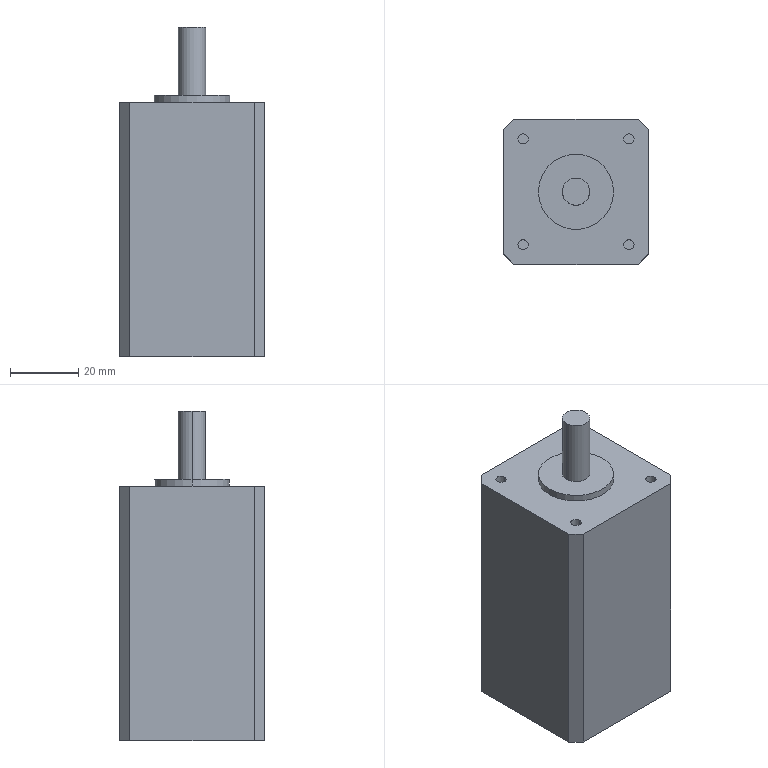Part | SolidWorks | features BaseBody 1 | 1 solid | 28 faces | box 42.3 x 42.3 x 96.5 mm | volume 133444 mm3 | plane 16 | cylinder 12 | commonest cylinder face diameters 3 x8 8 x2 22 x2
STEP:
#1=CARTESIAN_POINT('',(-11.,0.,76.5));
#2=VERTEX_POINT('',#1);
#3=CARTESIAN_POINT('',(11.,0.,76.5));
#4=VERTEX_POINT('',#3);
#5=CARTESIAN_POINT('',(0.,0.,76.5));
#6=DIRECTION('',(0.,0.,-1.));
#7=DIRECTION('',(-1.,0.,0.));
#8=AXIS2_PLACEMENT_3D('',#5,#6,#7);
#9=CIRCLE('',#8,11.);
#10=EDGE_CURVE('',#2,#4,#9,.T.);
#11=ORIENTED_EDGE('',*,*,#10,.T.);
#12=CARTESIAN_POINT('',(11.,0.,74.5));
#13=VERTEX_POINT('',#12);
#14=CARTESIAN_POINT('',(11.,0.,76.5));
#15=DIRECTION('',(0.,0.,-1.));
#16=VECTOR('',#15,1000.);
#17=LINE('',#14,#16);
#18=EDGE_CURVE('',#4,#13,#17,.T.);
#19=ORIENTED_EDGE('',*,*,#18,.T.);
#20=CARTESIAN_POINT('',(-11.,0.,74.5));
#21=VERTEX_POINT('',#20);
#22=CARTESIAN_POINT('',(0.,0.,74.5));
#23=DIRECTION('',(0.,0.,-1.));
#24=DIRECTION('',(-1.,0.,0.));
#25=AXIS2_PLACEMENT_3D('',#22,#23,#24);
#26=CIRCLE('',#25,11.);
#27=EDGE_CURVE('',#21,#13,#26,.T.);
#28=ORIENTED_EDGE('',*,*,#27,.F.);
#29=CARTESIAN_POINT('',(-11.,0.,76.5));
#30=DIRECTION('',(0.,0.,-1.));
#31=VECTOR('',#30,1000.);
#32=LINE('',#29,#31);
#33=EDGE_CURVE('',#2,#21,#32,.T.);
#34=ORIENTED_EDGE('',*,*,#33,.F.);
#35=EDGE_LOOP('',(#11,#19,#28,#34));
#36=FACE_OUTER_BOUND('',#35,.T.);
#37=CARTESIAN_POINT('',(0.,0.,76.5));
#38=DIRECTION('',(0.,0.,-1.));
#39=DIRECTION('',(-1.,0.,0.));
#40=AXIS2_PLACEMENT_3D('',#37,#38,#39);
#41=CYLINDRICAL_SURFACE('',#40,11.);
#42=ADVANCED_FACE('',(#36),#41,.T.);
#43=CARTESIAN_POINT('',(14.,-15.5,64.5));
#44=VERTEX_POINT('',#43);
#45=CARTESIAN_POINT('',(17.,-15.5,64.5));
#46=VERTEX_POINT('',#45);
#47=CARTESIAN_POINT('',(15.5,-15.5,64.5));
#48=DIRECTION('',(0.,0.,1.));
#49=DIRECTION('',(1.,0.,0.));
#50=AXIS2_PLACEMENT_3D('',#47,#48,#49);
#51=CIRCLE('',#50,1.5);
#52=EDGE_CURVE('',#44,#46,#51,.T.);
#53=ORIENTED_EDGE('',*,*,#52,.F.);
#54=CARTESIAN_POINT('',(14.,-15.5,74.5));
#55=VERTEX_POINT('',#54);
#56=CARTESIAN_POINT('',(14.,-15.5,64.5));
#57=DIRECTION('',(0.,0.,1.));
#58=VECTOR('',#57,1000.);
#59=LINE('',#56,#58);
#60=EDGE_CURVE('',#44,#55,#59,.T.);
#61=ORIENTED_EDGE('',*,*,#60,.T.);
#62=CARTESIAN_POINT('',(17.,-15.5,74.5));
#63=VERTEX_POINT('',#62);
#64=CARTESIAN_POINT('',(15.5,-15.5,74.5));
#65=DIRECTION('',(0.,0.,-1.));
#66=DIRECTION('',(1.,0.,0.));
#67=AXIS2_PLACEMENT_3D('',#64,#65,#66);
#68=CIRCLE('',#67,1.5);
#69=EDGE_CURVE('',#63,#55,#68,.T.);
#70=ORIENTED_EDGE('',*,*,#69,.F.);
#71=CARTESIAN_POINT('',(17.,-15.5,64.5));
#72=DIRECTION('',(0.,0.,1.));
#73=VECTOR('',#72,1000.);
#74=LINE('',#71,#73);
#75=EDGE_CURVE('',#46,#63,#74,.T.);
#76=ORIENTED_EDGE('',*,*,#75,.F.);
#77=EDGE_LOOP('',(#53,#61,#70,#76));
#78=FACE_OUTER_BOUND('',#77,.T.);
#79=CARTESIAN_POINT('',(15.5,-15.5,64.5));
#80=DIRECTION('',(0.,0.,1.));
#81=DIRECTION('',(1.,0.,0.));
#82=AXIS2_PLACEMENT_3D('',#79,#80,#81);
#83=CYLINDRICAL_SURFACE('',#82,1.5);
#84=ADVANCED_FACE('',(#78),#83,.F.);
#85=CARTESIAN_POINT('',(-17.,15.5,64.5));
#86=VERTEX_POINT('',#85);
#87=CARTESIAN_POINT('',(-14.,15.5,64.5));
#88=VERTEX_POINT('',#87);
#89=CARTESIAN_POINT('',(-15.5,15.5,64.5));
#90=DIRECTION('',(0.,0.,1.));
#91=DIRECTION('',(1.,0.,0.));
#92=AXIS2_PLACEMENT_3D('',#89,#90,#91);
#93=CIRCLE('',#92,1.5);
#94=EDGE_CURVE('',#86,#88,#93,.T.);
#95=ORIENTED_EDGE('',*,*,#94,.F.);
#96=CARTESIAN_POINT('',(-17.,15.5,74.5));
#97=VERTEX_POINT('',#96);
#98=CARTESIAN_POINT('',(-17.,15.5,64.5));
#99=DIRECTION('',(0.,0.,1.));
#100=VECTOR('',#99,1000.);
#101=LINE('',#98,#100);
#102=EDGE_CURVE('',#86,#97,#101,.T.);
#103=ORIENTED_EDGE('',*,*,#102,.T.);
#104=CARTESIAN_POINT('',(-14.,15.5,74.5));
#105=VERTEX_POINT('',#104);
#106=CARTESIAN_POINT('',(-15.5,15.5,74.5));
#107=DIRECTION('',(0.,0.,-1.));
#108=DIRECTION('',(1.,0.,0.));
#109=AXIS2_PLACEMENT_3D('',#106,#107,#108);
#110=CIRCLE('',#109,1.5);
#111=EDGE_CURVE('',#105,#97,#110,.T.);
#112=ORIENTED_EDGE('',*,*,#111,.F.);
#113=CARTESIAN_POINT('',(-14.,15.5,64.5));
#114=DIRECTION('',(0.,0.,1.));
#115=VECTOR('',#114,1000.);
#116=LINE('',#113,#115);
#117=EDGE_CURVE('',#88,#105,#116,.T.);
#118=ORIENTED_EDGE('',*,*,#117,.F.);
#119=EDGE_LOOP('',(#95,#103,#112,#118));
#120=FACE_OUTER_BOUND('',#119,.T.);
#121=CARTESIAN_POINT('',(-15.5,15.5,64.5));
#122=DIRECTION('',(0.,0.,1.));
#123=DIRECTION('',(1.,0.,0.));
#124=AXIS2_PLACEMENT_3D('',#121,#122,#123);
#125=CYLINDRICAL_SURFACE('',#124,1.5);
#126=ADVANCED_FACE('',(#120),#125,.F.);
#127=CARTESIAN_POINT('',(14.,15.5,64.5));
#128=VERTEX_POINT('',#127);
#129=CARTESIAN_POINT('',(17.,15.5,64.5));
#130=VERTEX_POINT('',#129);
#131=CARTESIAN_POINT('',(15.5,15.5,64.5));
#132=DIRECTION('',(0.,0.,1.));
#133=DIRECTION('',(1.,0.,0.));
#134=AXIS2_PLACEMENT_3D('',#131,#132,#133);
#135=CIRCLE('',#134,1.5);
#136=EDGE_CURVE('',#128,#130,#135,.T.);
#137=ORIENTED_EDGE('',*,*,#136,.F.);
#138=CARTESIAN_POINT('',(14.,15.5,74.5));
#139=VERTEX_POINT('',#138);
#140=CARTESIAN_POINT('',(14.,15.5,64.5));
#141=DIRECTION('',(0.,0.,1.));
#142=VECTOR('',#141,1000.);
#143=LINE('',#140,#142);
#144=EDGE_CURVE('',#128,#139,#143,.T.);
#145=ORIENTED_EDGE('',*,*,#144,.T.);
#146=CARTESIAN_POINT('',(17.,15.5,74.5));
#147=VERTEX_POINT('',#146);
#148=CARTESIAN_POINT('',(15.5,15.5,74.5));
#149=DIRECTION('',(0.,0.,-1.));
#150=DIRECTION('',(1.,0.,0.));
#151=AXIS2_PLACEMENT_3D('',#148,#149,#150);
#152=CIRCLE('',#151,1.5);
#153=EDGE_CURVE('',#147,#139,#152,.T.);
#154=ORIENTED_EDGE('',*,*,#153,.F.);
#155=CARTESIAN_POINT('',(17.,15.5,64.5));
#156=DIRECTION('',(0.,0.,1.));
#157=VECTOR('',#156,1000.);
#158=LINE('',#155,#157);
#159=EDGE_CURVE('',#130,#147,#158,.T.);
#160=ORIENTED_EDGE('',*,*,#159,.F.);
#161=EDGE_LOOP('',(#137,#145,#154,#160));
#162=FACE_OUTER_BOUND('',#161,.T.);
#163=CARTESIAN_POINT('',(15.5,15.5,64.5));
#164=DIRECTION('',(0.,0.,1.));
#165=DIRECTION('',(1.,0.,0.));
#166=AXIS2_PLACEMENT_3D('',#163,#164,#165);
#167=CYLINDRICAL_SURFACE('',#166,1.5);
#168=ADVANCED_FACE('',(#162),#167,.F.);
#169=CARTESIAN_POINT('',(-17.,-15.5,64.5));
#170=VERTEX_POINT('',#169);
#171=CARTESIAN_POINT('',(-14.,-15.5,64.5));
#172=VERTEX_POINT('',#171);
#173=CARTESIAN_POINT('',(-15.5,-15.5,64.5));
#174=DIRECTION('',(0.,0.,1.));
#175=DIRECTION('',(1.,0.,0.));
#176=AXIS2_PLACEMENT_3D('',#173,#174,#175);
#177=CIRCLE('',#176,1.5);
#178=EDGE_CURVE('',#170,#172,#177,.T.);
#179=ORIENTED_EDGE('',*,*,#178,.F.);
#180=CARTESIAN_POINT('',(-17.,-15.5,74.5));
#181=VERTEX_POINT('',#180);
#182=CARTESIAN_POINT('',(-17.,-15.5,64.5));
#183=DIRECTION('',(0.,0.,1.));
#184=VECTOR('',#183,1000.);
#185=LINE('',#182,#184);
#186=EDGE_CURVE('',#170,#181,#185,.T.);
#187=ORIENTED_EDGE('',*,*,#186,.T.);
#188=CARTESIAN_POINT('',(-14.,-15.5,74.5));
#189=VERTEX_POINT('',#188);
#190=CARTESIAN_POINT('',(-15.5,-15.5,74.5));
#191=DIRECTION('',(0.,0.,-1.));
#192=DIRECTION('',(1.,0.,0.));
#193=AXIS2_PLACEMENT_3D('',#190,#191,#192);
#194=CIRCLE('',#193,1.5);
#195=EDGE_CURVE('',#189,#181,#194,.T.);
#196=ORIENTED_EDGE('',*,*,#195,.F.);
#197=CARTESIAN_POINT('',(-14.,-15.5,64.5));
#198=DIRECTION('',(0.,0.,1.));
#199=VECTOR('',#198,1000.);
#200=LINE('',#197,#199);
#201=EDGE_CURVE('',#172,#189,#200,.T.);
#202=ORIENTED_EDGE('',*,*,#201,.F.);
#203=EDGE_LOOP('',(#179,#187,#196,#202));
#204=FACE_OUTER_BOUND('',#203,.T.);
#205=CARTESIAN_POINT('',(-15.5,-15.5,64.5));
#206=DIRECTION('',(0.,0.,1.));
#207=DIRECTION('',(1.,0.,0.));
#208=AXIS2_PLACEMENT_3D('',#205,#206,#207);
#209=CYLINDRICAL_SURFACE('',#208,1.5);
#210=ADVANCED_FACE('',(#204),#209,.F.);
#211=CARTESIAN_POINT('',(-4.,0.,96.5));
#212=VERTEX_POINT('',#211);
#213=CARTESIAN_POINT('',(4.,0.,96.5));
#214=VERTEX_POINT('',#213);
#215=CARTESIAN_POINT('',(0.,0.,96.5));
#216=DIRECTION('',(0.,0.,-1.));
#217=DIRECTION('',(-1.,0.,0.));
#218=AXIS2_PLACEMENT_3D('',#215,#216,#217);
#219=CIRCLE('',#218,4.);
#220=EDGE_CURVE('',#212,#214,#219,.T.);
#221=ORIENTED_EDGE('',*,*,#220,.T.);
#222=CARTESIAN_POINT('',(4.,0.,76.5));
#223=VERTEX_POINT('',#222);
#224=CARTESIAN_POINT('',(4.,0.,96.5));
#225=DIRECTION('',(0.,0.,-1.));
#226=VECTOR('',#225,1000.);
#227=LINE('',#224,#226);
#228=EDGE_CURVE('',#214,#223,#227,.T.);
#229=ORIENTED_EDGE('',*,*,#228,.T.);
#230=CARTESIAN_POINT('',(-4.,0.,76.5));
#231=VERTEX_POINT('',#230);
#232=CARTESIAN_POINT('',(0.,0.,76.5));
#233=DIRECTION('',(0.,0.,-1.));
#234=DIRECTION('',(-1.,0.,0.));
#235=AXIS2_PLACEMENT_3D('',#232,#233,#234);
#236=CIRCLE('',#235,4.);
#237=EDGE_CURVE('',#231,#223,#236,.T.);
#238=ORIENTED_EDGE('',*,*,#237,.F.);
#239=CARTESIAN_POINT('',(-4.,0.,96.5));
#240=DIRECTION('',(0.,0.,-1.));
#241=VECTOR('',#240,1000.);
#242=LINE('',#239,#241);
#243=EDGE_CURVE('',#212,#231,#242,.T.);
#244=ORIENTED_EDGE('',*,*,#243,.F.);
#245=EDGE_LOOP('',(#221,#229,#238,#244));
#246=FACE_OUTER_BOUND('',#245,.T.);
#247=CARTESIAN_POINT('',(0.,0.,96.5));
#248=DIRECTION('',(0.,0.,-1.));
#249=DIRECTION('',(-1.,0.,0.));
#250=AXIS2_PLACEMENT_3D('',#247,#248,#249);
#251=CYLINDRICAL_SURFACE('',#250,4.);
#252=ADVANCED_FACE('',(#246),#251,.T.);
#253=CARTESIAN_POINT('',(18.15,21.15,0.));
#254=VERTEX_POINT('',#253);
#255=CARTESIAN_POINT('',(18.15,21.15,74.5));
#256=VERTEX_POINT('',#255);
#257=CARTESIAN_POINT('',(18.15,21.15,74.5));
#258=DIRECTION('',(0.,0.,1.));
#259=VECTOR('',#258,1000.);
#260=LINE('',#257,#259);
#261=EDGE_CURVE('',#254,#256,#260,.T.);
#262=ORIENTED_EDGE('',*,*,#261,.F.);
#263=CARTESIAN_POINT('',(-18.15,21.15,0.));
#264=VERTEX_POINT('',#263);
#265=CARTESIAN_POINT('',(-21.15,21.15,0.));
#266=DIRECTION('',(1.,0.,0.));
#267=VECTOR('',#266,1000.);
#268=LINE('',#265,#267);
#269=EDGE_CURVE('',#264,#254,#268,.T.);
#270=ORIENTED_EDGE('',*,*,#269,.F.);
#271=CARTESIAN_POINT('',(-18.15,21.15,74.5));
#272=VERTEX_POINT('',#271);
#273=CARTESIAN_POINT('',(-18.15,21.15,74.5));
#274=DIRECTION('',(0.,0.,-1.));
#275=VECTOR('',#274,1000.);
#276=LINE('',#273,#275);
#277=EDGE_CURVE('',#272,#264,#276,.T.);
#278=ORIENTED_EDGE('',*,*,#277,.F.);
#279=CARTESIAN_POINT('',(-21.15,21.15,74.5));
#280=DIRECTION('',(-1.,0.,0.));
#281=VECTOR('',#280,1000.);
#282=LINE('',#279,#281);
#283=EDGE_CURVE('',#256,#272,#282,.T.);
#284=ORIENTED_EDGE('',*,*,#283,.F.);
#285=EDGE_LOOP('',(#262,#270,#278,#284));
#286=FACE_OUTER_BOUND('',#285,.T.);
#287=CARTESIAN_POINT('',(-21.15,21.15,74.5));
#288=DIRECTION('',(0.,-1.,0.));
#289=DIRECTION('',(0.,0.,-1.));
#290=AXIS2_PLACEMENT_3D('',#287,#288,#289);
#291=PLANE('',#290);
#292=ADVANCED_FACE('',(#286),#291,.F.);
#293=CARTESIAN_POINT('',(-18.15,-21.15,74.5));
#294=VERTEX_POINT('',#293);
#295=CARTESIAN_POINT('',(18.15,-21.15,74.5));
#296=VERTEX_POINT('',#295);
#297=CARTESIAN_POINT('',(0.,-21.15,74.5));
#298=DIRECTION('',(1.,0.,0.));
#299=VECTOR('',#298,1000.);
#300=LINE('',#297,#299);
#301=EDGE_CURVE('',#294,#296,#300,.T.);
#302=ORIENTED_EDGE('',*,*,#301,.T.);
#303=CARTESIAN_POINT('',(21.15,-18.15,74.5));
#304=VERTEX_POINT('',#303);
#305=CARTESIAN_POINT('',(18.15,-21.15,74.5));
#306=DIRECTION('',(0.7071,0.7071,0.));
#307=VECTOR('',#306,1000.);
#308=LINE('',#305,#307);
#309=EDGE_CURVE('',#296,#304,#308,.T.);
#310=ORIENTED_EDGE('',*,*,#309,.T.);
#311=CARTESIAN_POINT('',(21.15,18.15,74.5));
#312=VERTEX_POINT('',#311);
#313=CARTESIAN_POINT('',(21.15,0.,74.5));
#314=DIRECTION('',(0.,1.,0.));
#315=VECTOR('',#314,1000.);
#316=LINE('',#313,#315);
#317=EDGE_CURVE('',#304,#312,#316,.T.);
#318=ORIENTED_EDGE('',*,*,#317,.T.);
#319=CARTESIAN_POINT('',(21.15,18.15,74.5));
#320=DIRECTION('',(-0.7071,0.7071,0.));
#321=VECTOR('',#320,1000.);
#322=LINE('',#319,#321);
#323=EDGE_CURVE('',#312,#256,#322,.T.);
#324=ORIENTED_EDGE('',*,*,#323,.T.);
#325=ORIENTED_EDGE('',*,*,#283,.T.);
#326=CARTESIAN_POINT('',(-21.15,18.15,74.5));
#327=VERTEX_POINT('',#326);
#328=CARTESIAN_POINT('',(-18.15,21.15,74.5));
#329=DIRECTION('',(-0.7071,-0.7071,0.));
#330=VECTOR('',#329,1000.);
#331=LINE('',#328,#330);
#332=EDGE_CURVE('',#272,#327,#331,.T.);
#333=ORIENTED_EDGE('',*,*,#332,.T.);
#334=CARTESIAN_POINT('',(-21.15,-18.15,74.5));
#335=VERTEX_POINT('',#334);
#336=CARTESIAN_POINT('',(-21.15,0.,74.5));
#337=DIRECTION('',(0.,-1.,0.));
#338=VECTOR('',#337,1000.);
#339=LINE('',#336,#338);
#340=EDGE_CURVE('',#327,#335,#339,.T.);
#341=ORIENTED_EDGE('',*,*,#340,.T.);
#342=CARTESIAN_POINT('',(-21.15,-18.15,74.5));
#343=DIRECTION('',(0.7071,-0.7071,0.));
#344=VECTOR('',#343,1000.);
#345=LINE('',#342,#344);
#346=EDGE_CURVE('',#335,#294,#345,.T.);
#347=ORIENTED_EDGE('',*,*,#346,.T.);
#348=EDGE_LOOP('',(#302,#310,#318,#324,#325,#333,#341,#347));
#349=FACE_OUTER_BOUND('',#348,.T.);
#350=ORIENTED_EDGE('',*,*,#27,.T.);
#351=CARTESIAN_POINT('',(0.,0.,74.5));
#352=DIRECTION('',(0.,0.,-1.));
#353=DIRECTION('',(-1.,0.,0.));
#354=AXIS2_PLACEMENT_3D('',#351,#352,#353);
#355=CIRCLE('',#354,11.);
#356=EDGE_CURVE('',#13,#21,#355,.T.);
#357=ORIENTED_EDGE('',*,*,#356,.T.);
#358=EDGE_LOOP('',(#350,#357));
#359=FACE_BOUND('',#358,.T.);
#360=ORIENTED_EDGE('',*,*,#69,.T.);
#361=CARTESIAN_POINT('',(15.5,-15.5,74.5));
#362=DIRECTION('',(0.,0.,-1.));
#363=DIRECTION('',(1.,0.,0.));
#364=AXIS2_PLACEMENT_3D('',#361,#362,#363);
#365=CIRCLE('',#364,1.5);
#366=EDGE_CURVE('',#55,#63,#365,.T.);
#367=ORIENTED_EDGE('',*,*,#366,.T.);
#368=EDGE_LOOP('',(#360,#367));
#369=FACE_BOUND('',#368,.T.);
#370=ORIENTED_EDGE('',*,*,#111,.T.);
#371=CARTESIAN_POINT('',(-15.5,15.5,74.5));
#372=DIRECTION('',(0.,0.,-1.));
#373=DIRECTION('',(1.,0.,0.));
#374=AXIS2_PLACEMENT_3D('',#371,#372,#373);
#375=CIRCLE('',#374,1.5);
#376=EDGE_CURVE('',#97,#105,#375,.T.);
#377=ORIENTED_EDGE('',*,*,#376,.T.);
#378=EDGE_LOOP('',(#370,#377));
#379=FACE_BOUND('',#378,.T.);
#380=ORIENTED_EDGE('',*,*,#153,.T.);
#381=CARTESIAN_POINT('',(15.5,15.5,74.5));
#382=DIRECTION('',(0.,0.,-1.));
#383=DIRECTION('',(1.,0.,0.));
#384=AXIS2_PLACEMENT_3D('',#381,#382,#383);
#385=CIRCLE('',#384,1.5);
#386=EDGE_CURVE('',#139,#147,#385,.T.);
#387=ORIENTED_EDGE('',*,*,#386,.T.);
#388=EDGE_LOOP('',(#380,#387));
#389=FACE_BOUND('',#388,.T.);
#390=ORIENTED_EDGE('',*,*,#195,.T.);
#391=CARTESIAN_POINT('',(-15.5,-15.5,74.5));
#392=DIRECTION('',(0.,0.,-1.));
#393=DIRECTION('',(1.,0.,0.));
#394=AXIS2_PLACEMENT_3D('',#391,#392,#393);
#395=CIRCLE('',#394,1.5);
#396=EDGE_CURVE('',#181,#189,#395,.T.);
#397=ORIENTED_EDGE('',*,*,#396,.T.);
#398=EDGE_LOOP('',(#390,#397));
#399=FACE_BOUND('',#398,.T.);
#400=CARTESIAN_POINT('',(0.,0.,74.5));
#401=DIRECTION('',(0.,0.,1.));
#402=DIRECTION('',(1.,0.,0.));
#403=AXIS2_PLACEMENT_3D('',#400,#401,#402);
#404=PLANE('',#403);
#405=ADVANCED_FACE('',(#349,#359,#369,#379,#389,#399),#404,.T.);
#406=CARTESIAN_POINT('',(21.15,18.15,0.));
#407=VERTEX_POINT('',#406);
#408=CARTESIAN_POINT('',(21.15,18.15,74.5));
#409=DIRECTION('',(0.,0.,1.));
#410=VECTOR('',#409,1000.);
#411=LINE('',#408,#410);
#412=EDGE_CURVE('',#407,#312,#411,.T.);
#413=ORIENTED_EDGE('',*,*,#412,.F.);
#414=CARTESIAN_POINT('',(18.15,21.15,0.));
#415=DIRECTION('',(0.7071,-0.7071,0.));
#416=VECTOR('',#415,1000.);
#417=LINE('',#414,#416);
#418=EDGE_CURVE('',#254,#407,#417,.T.);
#419=ORIENTED_EDGE('',*,*,#418,.F.);
#420=ORIENTED_EDGE('',*,*,#261,.T.);
#421=ORIENTED_EDGE('',*,*,#323,.F.);
#422=EDGE_LOOP('',(#413,#419,#420,#421));
#423=FACE_OUTER_BOUND('',#422,.T.);
#424=CARTESIAN_POINT('',(18.15,21.15,74.5));
#425=DIRECTION('',(-0.7071,-0.7071,0.));
#426=DIRECTION('',(0.7071,-0.7071,0.));
#427=AXIS2_PLACEMENT_3D('',#424,#425,#426);
#428=PLANE('',#427);
#429=ADVANCED_FACE('',(#423),#428,.F.);
#430=ORIENTED_EDGE('',*,*,#418,.T.);
#431=CARTESIAN_POINT('',(21.15,-18.15,0.));
#432=VERTEX_POINT('',#431);
#433=CARTESIAN_POINT('',(21.15,0.,0.));
#434=DIRECTION('',(0.,1.,0.));
#435=VECTOR('',#434,1000.);
#436=LINE('',#433,#435);
#437=EDGE_CURVE('',#432,#407,#436,.T.);
#438=ORIENTED_EDGE('',*,*,#437,.F.);
#439=CARTESIAN_POINT('',(18.15,-21.15,0.));
#440=VERTEX_POINT('',#439);
#441=CARTESIAN_POINT('',(18.15,-21.15,0.));
#442=DIRECTION('',(0.7071,0.7071,0.));
#443=VECTOR('',#442,1000.);
#444=LINE('',#441,#443);
#445=EDGE_CURVE('',#440,#432,#444,.T.);
#446=ORIENTED_EDGE('',*,*,#445,.F.);
#447=CARTESIAN_POINT('',(-18.15,-21.15,0.));
#448=VERTEX_POINT('',#447);
#449=CARTESIAN_POINT('',(0.,-21.15,0.));
#450=DIRECTION('',(1.,0.,0.));
#451=VECTOR('',#450,1000.);
#452=LINE('',#449,#451);
#453=EDGE_CURVE('',#448,#440,#452,.T.);
#454=ORIENTED_EDGE('',*,*,#453,.F.);
#455=CARTESIAN_POINT('',(-21.15,-18.15,0.));
#456=VERTEX_POINT('',#455);
#457=CARTESIAN_POINT('',(-21.15,-18.15,0.));
#458=DIRECTION('',(0.7071,-0.7071,0.));
#459=VECTOR('',#458,1000.);
#460=LINE('',#457,#459);
#461=EDGE_CURVE('',#456,#448,#460,.T.);
#462=ORIENTED_EDGE('',*,*,#461,.F.);
#463=CARTESIAN_POINT('',(-21.15,18.15,0.));
#464=VERTEX_POINT('',#463);
#465=CARTESIAN_POINT('',(-21.15,0.,0.));
#466=DIRECTION('',(0.,-1.,0.));
#467=VECTOR('',#466,1000.);
#468=LINE('',#465,#467);
#469=EDGE_CURVE('',#464,#456,#468,.T.);
#470=ORIENTED_EDGE('',*,*,#469,.F.);
#471=CARTESIAN_POINT('',(-18.15,21.15,0.));
#472=DIRECTION('',(-0.7071,-0.7071,0.));
#473=VECTOR('',#472,1000.);
#474=LINE('',#471,#473);
#475=EDGE_CURVE('',#264,#464,#474,.T.);
#476=ORIENTED_EDGE('',*,*,#475,.F.);
#477=ORIENTED_EDGE('',*,*,#269,.T.);
#478=EDGE_LOOP('',(#430,#438,#446,#454,#462,#470,#476,#477));
#479=FACE_OUTER_BOUND('',#478,.T.);
#480=CARTESIAN_POINT('',(0.,0.,0.));
#481=DIRECTION('',(0.,0.,1.));
#482=DIRECTION('',(1.,0.,0.));
#483=AXIS2_PLACEMENT_3D('',#480,#481,#482);
#484=PLANE('',#483);
#485=ADVANCED_FACE('',(#479),#484,.F.);
#486=ORIENTED_EDGE('',*,*,#277,.T.);
#487=ORIENTED_EDGE('',*,*,#475,.T.);
#488=CARTESIAN_POINT('',(-21.15,18.15,74.5));
#489=DIRECTION('',(0.,0.,-1.));
#490=VECTOR('',#489,1000.);
#491=LINE('',#488,#490);
#492=EDGE_CURVE('',#327,#464,#491,.T.);
#493=ORIENTED_EDGE('',*,*,#492,.F.);
#494=ORIENTED_EDGE('',*,*,#332,.F.);
#495=EDGE_LOOP('',(#486,#487,#493,#494));
#496=FACE_OUTER_BOUND('',#495,.T.);
#497=CARTESIAN_POINT('',(-21.15,18.15,74.5));
#498=DIRECTION('',(0.7071,-0.7071,0.));
#499=DIRECTION('',(0.7071,0.7071,0.));
#500=AXIS2_PLACEMENT_3D('',#497,#498,#499);
#501=PLANE('',#500);
#502=ADVANCED_FACE('',(#496),#501,.F.);
#503=CARTESIAN_POINT('',(18.15,-21.15,74.5));
#504=DIRECTION('',(0.,0.,1.));
#505=VECTOR('',#504,1000.);
#506=LINE('',#503,#505);
#507=EDGE_CURVE('',#440,#296,#506,.T.);
#508=ORIENTED_EDGE('',*,*,#507,.F.);
#509=ORIENTED_EDGE('',*,*,#445,.T.);
#510=CARTESIAN_POINT('',(21.15,-18.15,74.5));
#511=DIRECTION('',(0.,0.,-1.));
#512=VECTOR('',#511,1000.);
#513=LINE('',#510,#512);
#514=EDGE_CURVE('',#304,#432,#513,.T.);
#515=ORIENTED_EDGE('',*,*,#514,.F.);
#516=ORIENTED_EDGE('',*,*,#309,.F.);
#517=EDGE_LOOP('',(#508,#509,#515,#516));
#518=FACE_OUTER_BOUND('',#517,.T.);
#519=CARTESIAN_POINT('',(21.15,-18.15,74.5));
#520=DIRECTION('',(-0.7071,0.7071,0.));
#521=DIRECTION('',(-0.7071,-0.7071,0.));
#522=AXIS2_PLACEMENT_3D('',#519,#520,#521);
#523=PLANE('',#522);
#524=ADVANCED_FACE('',(#518),#523,.F.);
#525=ORIENTED_EDGE('',*,*,#507,.T.);
#526=ORIENTED_EDGE('',*,*,#301,.F.);
#527=CARTESIAN_POINT('',(-18.15,-21.15,74.5));
#528=DIRECTION('',(0.,0.,1.));
#529=VECTOR('',#528,1000.);
#530=LINE('',#527,#529);
#531=EDGE_CURVE('',#448,#294,#530,.T.);
#532=ORIENTED_EDGE('',*,*,#531,.F.);
#533=ORIENTED_EDGE('',*,*,#453,.T.);
#534=EDGE_LOOP('',(#525,#526,#532,#533));
#535=FACE_OUTER_BOUND('',#534,.T.);
#536=CARTESIAN_POINT('',(-21.15,-21.15,74.5));
#537=DIRECTION('',(0.,1.,0.));
#538=DIRECTION('',(0.,0.,1.));
#539=AXIS2_PLACEMENT_3D('',#536,#537,#538);
#540=PLANE('',#539);
#541=ADVANCED_FACE('',(#535),#540,.F.);
#542=CARTESIAN_POINT('',(-21.15,-18.15,74.5));
#543=DIRECTION('',(0.,0.,1.));
#544=VECTOR('',#543,1000.);
#545=LINE('',#542,#544);
#546=EDGE_CURVE('',#456,#335,#545,.T.);
#547=ORIENTED_EDGE('',*,*,#546,.F.);
#548=ORIENTED_EDGE('',*,*,#461,.T.);
#549=ORIENTED_EDGE('',*,*,#531,.T.);
#550=ORIENTED_EDGE('',*,*,#346,.F.);
#551=EDGE_LOOP('',(#547,#548,#549,#550));
#552=FACE_OUTER_BOUND('',#551,.T.);
#553=CARTESIAN_POINT('',(-18.15,-21.15,74.5));
#554=DIRECTION('',(0.7071,0.7071,0.));
#555=DIRECTION('',(-0.7071,0.7071,0.));
#556=AXIS2_PLACEMENT_3D('',#553,#554,#555);
#557=PLANE('',#556);
#558=ADVANCED_FACE('',(#552),#557,.F.);
#559=ORIENTED_EDGE('',*,*,#492,.T.);
#560=ORIENTED_EDGE('',*,*,#469,.T.);
#561=ORIENTED_EDGE('',*,*,#546,.T.);
#562=ORIENTED_EDGE('',*,*,#340,.F.);
#563=EDGE_LOOP('',(#559,#560,#561,#562));
#564=FACE_OUTER_BOUND('',#563,.T.);
#565=CARTESIAN_POINT('',(-21.15,21.15,74.5));
#566=DIRECTION('',(1.,0.,0.));
#567=DIRECTION('',(0.,1.,0.));
#568=AXIS2_PLACEMENT_3D('',#565,#566,#567);
#569=PLANE('',#568);
#570=ADVANCED_FACE('',(#564),#569,.F.);
#571=ORIENTED_EDGE('',*,*,#412,.T.);
#572=ORIENTED_EDGE('',*,*,#317,.F.);
#573=ORIENTED_EDGE('',*,*,#514,.T.);
#574=ORIENTED_EDGE('',*,*,#437,.T.);
#575=EDGE_LOOP('',(#571,#572,#573,#574));
#576=FACE_OUTER_BOUND('',#575,.T.);
#577=CARTESIAN_POINT('',(21.15,21.15,74.5));
#578=DIRECTION('',(-1.,0.,0.));
#579=DIRECTION('',(0.,-1.,0.));
#580=AXIS2_PLACEMENT_3D('',#577,#578,#579);
#581=PLANE('',#580);
#582=ADVANCED_FACE('',(#576),#581,.F.);
#583=ORIENTED_EDGE('',*,*,#18,.F.);
#584=CARTESIAN_POINT('',(0.,0.,76.5));
#585=DIRECTION('',(0.,0.,-1.));
#586=DIRECTION('',(-1.,0.,0.));
#587=AXIS2_PLACEMENT_3D('',#584,#585,#586);
#588=CIRCLE('',#587,11.);
#589=EDGE_CURVE('',#4,#2,#588,.T.);
#590=ORIENTED_EDGE('',*,*,#589,.T.);
#591=ORIENTED_EDGE('',*,*,#33,.T.);
#592=ORIENTED_EDGE('',*,*,#356,.F.);
#593=EDGE_LOOP('',(#583,#590,#591,#592));
#594=FACE_OUTER_BOUND('',#593,.T.);
#595=CARTESIAN_POINT('',(0.,0.,76.5));
#596=DIRECTION('',(0.,0.,-1.));
#597=DIRECTION('',(-1.,0.,0.));
#598=AXIS2_PLACEMENT_3D('',#595,#596,#597);
#599=CYLINDRICAL_SURFACE('',#598,11.);
#600=ADVANCED_FACE('',(#594),#599,.T.);
#601=ORIENTED_EDGE('',*,*,#60,.F.);
#602=CARTESIAN_POINT('',(15.5,-15.5,64.5));
#603=DIRECTION('',(0.,0.,1.));
#604=DIRECTION('',(1.,0.,0.));
#605=AXIS2_PLACEMENT_3D('',#602,#603,#604);
#606=CIRCLE('',#605,1.5);
#607=EDGE_CURVE('',#46,#44,#606,.T.);
#608=ORIENTED_EDGE('',*,*,#607,.F.);
#609=ORIENTED_EDGE('',*,*,#75,.T.);
#610=ORIENTED_EDGE('',*,*,#366,.F.);
#611=EDGE_LOOP('',(#601,#608,#609,#610));
#612=FACE_OUTER_BOUND('',#611,.T.);
#613=CARTESIAN_POINT('',(15.5,-15.5,64.5));
#614=DIRECTION('',(0.,0.,1.));
#615=DIRECTION('',(1.,0.,0.));
#616=AXIS2_PLACEMENT_3D('',#613,#614,#615);
#617=CYLINDRICAL_SURFACE('',#616,1.5);
#618=ADVANCED_FACE('',(#612),#617,.F.);
#619=ORIENTED_EDGE('',*,*,#102,.F.);
#620=CARTESIAN_POINT('',(-15.5,15.5,64.5));
#621=DIRECTION('',(0.,0.,1.));
#622=DIRECTION('',(1.,0.,0.));
#623=AXIS2_PLACEMENT_3D('',#620,#621,#622);
#624=CIRCLE('',#623,1.5);
#625=EDGE_CURVE('',#88,#86,#624,.T.);
#626=ORIENTED_EDGE('',*,*,#625,.F.);
#627=ORIENTED_EDGE('',*,*,#117,.T.);
#628=ORIENTED_EDGE('',*,*,#376,.F.);
#629=EDGE_LOOP('',(#619,#626,#627,#628));
#630=FACE_OUTER_BOUND('',#629,.T.);
#631=CARTESIAN_POINT('',(-15.5,15.5,64.5));
#632=DIRECTION('',(0.,0.,1.));
#633=DIRECTION('',(1.,0.,0.));
#634=AXIS2_PLACEMENT_3D('',#631,#632,#633);
#635=CYLINDRICAL_SURFACE('',#634,1.5);
#636=ADVANCED_FACE('',(#630),#635,.F.);
#637=ORIENTED_EDGE('',*,*,#144,.F.);
#638=CARTESIAN_POINT('',(15.5,15.5,64.5));
#639=DIRECTION('',(0.,0.,1.));
#640=DIRECTION('',(1.,0.,0.));
#641=AXIS2_PLACEMENT_3D('',#638,#639,#640);
#642=CIRCLE('',#641,1.5);
#643=EDGE_CURVE('',#130,#128,#642,.T.);
#644=ORIENTED_EDGE('',*,*,#643,.F.);
#645=ORIENTED_EDGE('',*,*,#159,.T.);
#646=ORIENTED_EDGE('',*,*,#386,.F.);
#647=EDGE_LOOP('',(#637,#644,#645,#646));
#648=FACE_OUTER_BOUND('',#647,.T.);
#649=CARTESIAN_POINT('',(15.5,15.5,64.5));
#650=DIRECTION('',(0.,0.,1.));
#651=DIRECTION('',(1.,0.,0.));
#652=AXIS2_PLACEMENT_3D('',#649,#650,#651);
#653=CYLINDRICAL_SURFACE('',#652,1.5);
#654=ADVANCED_FACE('',(#648),#653,.F.);
#655=ORIENTED_EDGE('',*,*,#186,.F.);
#656=CARTESIAN_POINT('',(-15.5,-15.5,64.5));
#657=DIRECTION('',(0.,0.,1.));
#658=DIRECTION('',(1.,0.,0.));
#659=AXIS2_PLACEMENT_3D('',#656,#657,#658);
#660=CIRCLE('',#659,1.5);
#661=EDGE_CURVE('',#172,#170,#660,.T.);
#662=ORIENTED_EDGE('',*,*,#661,.F.);
#663=ORIENTED_EDGE('',*,*,#201,.T.);
#664=ORIENTED_EDGE('',*,*,#396,.F.);
#665=EDGE_LOOP('',(#655,#662,#663,#664));
#666=FACE_OUTER_BOUND('',#665,.T.);
#667=CARTESIAN_POINT('',(-15.5,-15.5,64.5));
#668=DIRECTION('',(0.,0.,1.));
#669=DIRECTION('',(1.,0.,0.));
#670=AXIS2_PLACEMENT_3D('',#667,#668,#669);
#671=CYLINDRICAL_SURFACE('',#670,1.5);
#672=ADVANCED_FACE('',(#666),#671,.F.);
#673=ORIENTED_EDGE('',*,*,#10,.F.);
#674=ORIENTED_EDGE('',*,*,#589,.F.);
#675=EDGE_LOOP('',(#673,#674));
#676=FACE_OUTER_BOUND('',#675,.T.);
#677=ORIENTED_EDGE('',*,*,#237,.T.);
#678=CARTESIAN_POINT('',(0.,0.,76.5));
#679=DIRECTION('',(0.,0.,-1.));
#680=DIRECTION('',(-1.,0.,0.));
#681=AXIS2_PLACEMENT_3D('',#678,#679,#680);
#682=CIRCLE('',#681,4.);
#683=EDGE_CURVE('',#223,#231,#682,.T.);
#684=ORIENTED_EDGE('',*,*,#683,.T.);
#685=EDGE_LOOP('',(#677,#684));
#686=FACE_BOUND('',#685,.T.);
#687=CARTESIAN_POINT('',(0.,0.,76.5));
#688=DIRECTION('',(0.,0.,1.));
#689=DIRECTION('',(1.,0.,0.));
#690=AXIS2_PLACEMENT_3D('',#687,#688,#689);
#691=PLANE('',#690);
#692=ADVANCED_FACE('',(#676,#686),#691,.T.);
#693=ORIENTED_EDGE('',*,*,#607,.T.);
#694=ORIENTED_EDGE('',*,*,#52,.T.);
#695=EDGE_LOOP('',(#693,#694));
#696=FACE_OUTER_BOUND('',#695,.T.);
#697=CARTESIAN_POINT('',(15.5,-15.5,64.5));
#698=DIRECTION('',(0.,0.,1.));
#699=DIRECTION('',(1.,0.,0.));
#700=AXIS2_PLACEMENT_3D('',#697,#698,#699);
#701=PLANE('',#700);
#702=ADVANCED_FACE('',(#696),#701,.T.);
#703=ORIENTED_EDGE('',*,*,#625,.T.);
#704=ORIENTED_EDGE('',*,*,#94,.T.);
#705=EDGE_LOOP('',(#703,#704));
#706=FACE_OUTER_BOUND('',#705,.T.);
#707=CARTESIAN_POINT('',(-15.5,15.5,64.5));
#708=DIRECTION('',(0.,0.,1.));
#709=DIRECTION('',(1.,0.,0.));
#710=AXIS2_PLACEMENT_3D('',#707,#708,#709);
#711=PLANE('',#710);
#712=ADVANCED_FACE('',(#706),#711,.T.);
#713=ORIENTED_EDGE('',*,*,#643,.T.);
#714=ORIENTED_EDGE('',*,*,#136,.T.);
#715=EDGE_LOOP('',(#713,#714));
#716=FACE_OUTER_BOUND('',#715,.T.);
#717=CARTESIAN_POINT('',(15.5,15.5,64.5));
#718=DIRECTION('',(0.,0.,1.));
#719=DIRECTION('',(1.,0.,0.));
#720=AXIS2_PLACEMENT_3D('',#717,#718,#719);
#721=PLANE('',#720);
#722=ADVANCED_FACE('',(#716),#721,.T.);
#723=ORIENTED_EDGE('',*,*,#661,.T.);
#724=ORIENTED_EDGE('',*,*,#178,.T.);
#725=EDGE_LOOP('',(#723,#724));
#726=FACE_OUTER_BOUND('',#725,.T.);
#727=CARTESIAN_POINT('',(-15.5,-15.5,64.5));
#728=DIRECTION('',(0.,0.,1.));
#729=DIRECTION('',(1.,0.,0.));
#730=AXIS2_PLACEMENT_3D('',#727,#728,#729);
#731=PLANE('',#730);
#732=ADVANCED_FACE('',(#726),#731,.T.);
#733=ORIENTED_EDGE('',*,*,#228,.F.);
#734=CARTESIAN_POINT('',(0.,0.,96.5));
#735=DIRECTION('',(0.,0.,-1.));
#736=DIRECTION('',(-1.,0.,0.));
#737=AXIS2_PLACEMENT_3D('',#734,#735,#736);
#738=CIRCLE('',#737,4.);
#739=EDGE_CURVE('',#214,#212,#738,.T.);
#740=ORIENTED_EDGE('',*,*,#739,.T.);
#741=ORIENTED_EDGE('',*,*,#243,.T.);
#742=ORIENTED_EDGE('',*,*,#683,.F.);
#743=EDGE_LOOP('',(#733,#740,#741,#742));
#744=FACE_OUTER_BOUND('',#743,.T.);
#745=CARTESIAN_POINT('',(0.,0.,96.5));
#746=DIRECTION('',(0.,0.,-1.));
#747=DIRECTION('',(-1.,0.,0.));
#748=AXIS2_PLACEMENT_3D('',#745,#746,#747);
#749=CYLINDRICAL_SURFACE('',#748,4.);
#750=ADVANCED_FACE('',(#744),#749,.T.);
#751=ORIENTED_EDGE('',*,*,#220,.F.);
#752=ORIENTED_EDGE('',*,*,#739,.F.);
#753=EDGE_LOOP('',(#751,#752));
#754=FACE_OUTER_BOUND('',#753,.T.);
#755=CARTESIAN_POINT('',(0.,0.,96.5));
#756=DIRECTION('',(0.,0.,1.));
#757=DIRECTION('',(1.,0.,0.));
#758=AXIS2_PLACEMENT_3D('',#755,#756,#757);
#759=PLANE('',#758);
#760=ADVANCED_FACE('',(#754),#759,.T.);
#761=CLOSED_SHELL('',(#42,#84,#126,#168,#210,#252,#292,#405,#429,#485,#502,#524,#541,#558,#570,#582,#600,#618,#636,#654,#672,#692,#702,#712,#722,#732,#750,#760));
#762=MANIFOLD_SOLID_BREP('',#761);
#763=CARTESIAN_POINT('',(0.,0.,0.));
#764=DIRECTION('',(0.,0.,1.));
#765=DIRECTION('',(1.,0.,0.));
#766=AXIS2_PLACEMENT_3D('',#763,#764,#765);
#767=(LENGTH_UNIT()NAMED_UNIT(*)SI_UNIT(.MILLI.,.METRE.));
#768=UNCERTAINTY_MEASURE_WITH_UNIT(LENGTH_MEASURE(0.00001),#767,'','');
#769=(NAMED_UNIT(*)PLANE_ANGLE_UNIT()SI_UNIT($,.RADIAN.));
#770=(NAMED_UNIT(*)SI_UNIT($,.STERADIAN.)SOLID_ANGLE_UNIT());
#771=(GEOMETRIC_REPRESENTATION_CONTEXT(3)GLOBAL_UNCERTAINTY_ASSIGNED_CONTEXT((#768))GLOBAL_UNIT_ASSIGNED_CONTEXT((#767,#769,#770))REPRESENTATION_CONTEXT('',''));
#772=ADVANCED_BREP_SHAPE_REPRESENTATION('',(#762,#766),#771);